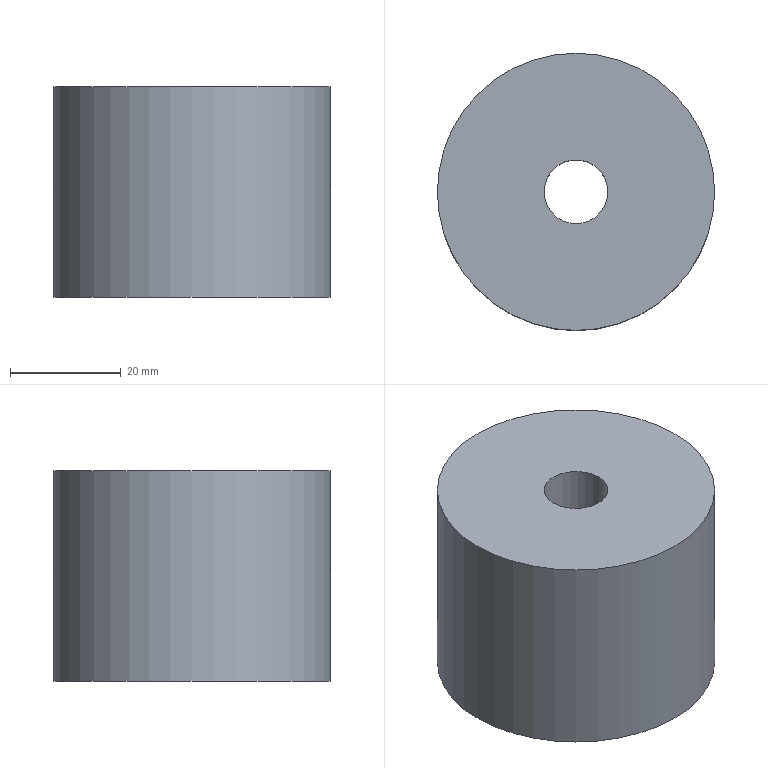Part | NX | features solid 2 | 1 solid | 6 faces | box 50 x 50 x 38 mm | volume 67952 mm3 | cylinder 3 | plane 3 | commonest cylinder face diameters 11.509 x1 18 x1 50 x1
STEP:
#1=CARTESIAN_POINT('',(1085.5,-230.,50.));
#2=VERTEX_POINT('',#1);
#3=CARTESIAN_POINT('',(1060.5,-230.,50.));
#4=DIRECTION('',(0.,0.,1.));
#5=DIRECTION('',(1.,0.,0.));
#6=AXIS2_PLACEMENT_3D('',#3,#4,#5);
#7=CIRCLE('',#6,25.);
#8=EDGE_CURVE('',#2,#2,#7,.T.);
#9=ORIENTED_EDGE('',*,*,#8,.T.);
#10=EDGE_LOOP('',(#9));
#11=FACE_BOUND('',#10,.T.);
#12=CARTESIAN_POINT('',(1085.5,-230.,88.));
#13=VERTEX_POINT('',#12);
#14=CARTESIAN_POINT('',(1060.5,-230.,88.));
#15=DIRECTION('',(0.,0.,-1.));
#16=DIRECTION('',(1.,0.,0.));
#17=AXIS2_PLACEMENT_3D('',#14,#15,#16);
#18=CIRCLE('',#17,25.);
#19=EDGE_CURVE('',#13,#13,#18,.T.);
#20=ORIENTED_EDGE('',*,*,#19,.T.);
#21=EDGE_LOOP('',(#20));
#22=FACE_BOUND('',#21,.T.);
#23=CARTESIAN_POINT('',(1060.5,-230.,20.));
#24=DIRECTION('',(0.,0.,-1.));
#25=DIRECTION('',(1.,0.,0.));
#26=AXIS2_PLACEMENT_3D('',#23,#24,#25);
#27=CYLINDRICAL_SURFACE('',#26,25.);
#28=ADVANCED_FACE('',(#11,#22),#27,.T.);
#29=CARTESIAN_POINT('',(1066.255,-230.,68.));
#30=VERTEX_POINT('',#29);
#31=CARTESIAN_POINT('',(1060.5,-230.,68.));
#32=DIRECTION('',(0.,0.,-1.));
#33=DIRECTION('',(1.,0.,0.));
#34=AXIS2_PLACEMENT_3D('',#31,#32,#33);
#35=CIRCLE('',#34,5.755);
#36=EDGE_CURVE('',#30,#30,#35,.F.);
#37=ORIENTED_EDGE('',*,*,#36,.F.);
#38=EDGE_LOOP('',(#37));
#39=FACE_BOUND('',#38,.T.);
#40=CARTESIAN_POINT('',(1066.255,-230.,88.));
#41=VERTEX_POINT('',#40);
#42=CARTESIAN_POINT('',(1060.5,-230.,88.));
#43=DIRECTION('',(0.,0.,-1.));
#44=DIRECTION('',(1.,0.,0.));
#45=AXIS2_PLACEMENT_3D('',#42,#43,#44);
#46=CIRCLE('',#45,5.755);
#47=EDGE_CURVE('',#41,#41,#46,.F.);
#48=ORIENTED_EDGE('',*,*,#47,.T.);
#49=EDGE_LOOP('',(#48));
#50=FACE_BOUND('',#49,.T.);
#51=CARTESIAN_POINT('',(1060.5,-230.,55.));
#52=DIRECTION('',(0.,0.,1.));
#53=DIRECTION('',(-1.,0.,0.));
#54=AXIS2_PLACEMENT_3D('',#51,#52,#53);
#55=CYLINDRICAL_SURFACE('',#54,5.755);
#56=ADVANCED_FACE('',(#39,#50),#55,.F.);
#57=CARTESIAN_POINT('',(1069.5,-230.,68.));
#58=VERTEX_POINT('',#57);
#59=CARTESIAN_POINT('',(1060.5,-230.,68.));
#60=DIRECTION('',(0.,0.,-1.));
#61=DIRECTION('',(1.,0.,0.));
#62=AXIS2_PLACEMENT_3D('',#59,#60,#61);
#63=CIRCLE('',#62,9.);
#64=EDGE_CURVE('',#58,#58,#63,.F.);
#65=ORIENTED_EDGE('',*,*,#64,.T.);
#66=EDGE_LOOP('',(#65));
#67=FACE_BOUND('',#66,.T.);
#68=CARTESIAN_POINT('',(1051.5,-230.,50.));
#69=VERTEX_POINT('',#68);
#70=CARTESIAN_POINT('',(1060.5,-230.,50.));
#71=DIRECTION('',(0.,0.,1.));
#72=DIRECTION('',(-1.,0.,0.));
#73=AXIS2_PLACEMENT_3D('',#70,#71,#72);
#74=CIRCLE('',#73,9.);
#75=EDGE_CURVE('',#69,#69,#74,.F.);
#76=ORIENTED_EDGE('',*,*,#75,.T.);
#77=EDGE_LOOP('',(#76));
#78=FACE_BOUND('',#77,.T.);
#79=CARTESIAN_POINT('',(1060.5,-230.,20.));
#80=DIRECTION('',(0.,0.,1.));
#81=DIRECTION('',(-1.,0.,0.));
#82=AXIS2_PLACEMENT_3D('',#79,#80,#81);
#83=CYLINDRICAL_SURFACE('',#82,9.);
#84=ADVANCED_FACE('',(#67,#78),#83,.F.);
#85=ORIENTED_EDGE('',*,*,#36,.T.);
#86=EDGE_LOOP('',(#85));
#87=FACE_BOUND('',#86,.T.);
#88=ORIENTED_EDGE('',*,*,#64,.F.);
#89=EDGE_LOOP('',(#88));
#90=FACE_BOUND('',#89,.T.);
#91=CARTESIAN_POINT('',(1060.5,-230.,68.));
#92=DIRECTION('',(0.,0.,1.));
#93=DIRECTION('',(-1.,0.,0.));
#94=AXIS2_PLACEMENT_3D('',#91,#92,#93);
#95=PLANE('',#94);
#96=ADVANCED_FACE('',(#87,#90),#95,.F.);
#97=ORIENTED_EDGE('',*,*,#75,.F.);
#98=EDGE_LOOP('',(#97));
#99=FACE_BOUND('',#98,.T.);
#100=ORIENTED_EDGE('',*,*,#8,.F.);
#101=EDGE_LOOP('',(#100));
#102=FACE_BOUND('',#101,.T.);
#103=CARTESIAN_POINT('',(722.5,25.,50.));
#104=DIRECTION('',(0.,0.,-1.));
#105=DIRECTION('',(1.,0.,0.));
#106=AXIS2_PLACEMENT_3D('',#103,#104,#105);
#107=PLANE('',#106);
#108=ADVANCED_FACE('',(#99,#102),#107,.T.);
#109=ORIENTED_EDGE('',*,*,#47,.F.);
#110=EDGE_LOOP('',(#109));
#111=FACE_BOUND('',#110,.T.);
#112=ORIENTED_EDGE('',*,*,#19,.F.);
#113=EDGE_LOOP('',(#112));
#114=FACE_BOUND('',#113,.T.);
#115=CARTESIAN_POINT('',(-321.121,140.,88.));
#116=DIRECTION('',(0.,0.,1.));
#117=DIRECTION('',(-1.,0.,0.));
#118=AXIS2_PLACEMENT_3D('',#115,#116,#117);
#119=PLANE('',#118);
#120=ADVANCED_FACE('',(#111,#114),#119,.T.);
#121=CLOSED_SHELL('',(#28,#56,#84,#96,#108,#120));
#122=MANIFOLD_SOLID_BREP('',#121);
#123=(LENGTH_UNIT()NAMED_UNIT(*)SI_UNIT(.MILLI.,.METRE.));
#124=UNCERTAINTY_MEASURE_WITH_UNIT(LENGTH_MEASURE(0.00001),#123,'','');
#125=(NAMED_UNIT(*)PLANE_ANGLE_UNIT()SI_UNIT($,.RADIAN.));
#126=(NAMED_UNIT(*)SI_UNIT($,.STERADIAN.)SOLID_ANGLE_UNIT());
#127=(GEOMETRIC_REPRESENTATION_CONTEXT(3)GLOBAL_UNCERTAINTY_ASSIGNED_CONTEXT((#124))GLOBAL_UNIT_ASSIGNED_CONTEXT((#123,#125,#126))REPRESENTATION_CONTEXT('',''));
#128=ADVANCED_BREP_SHAPE_REPRESENTATION('',(#122),#127);